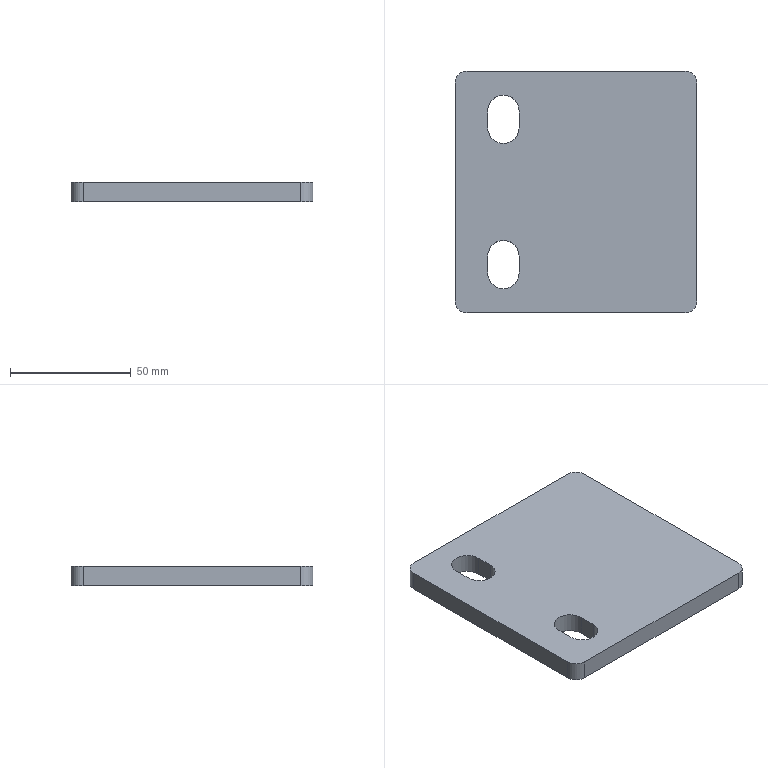Part | STEP file | HL4GD-1.30.104 cab frame rear mounting plate-
-20251212 | 1 solid | 18 faces | box 100 x 100 x 8 mm | volume 76249 mm3 | plane 10 | cylinder 8 | commonest cylinder face diameters 10 x4 13 x4
STEP:
#1=CARTESIAN_POINT('',(0.,0.,0.));
#2=DIRECTION('',(0.,0.,1.));
#3=DIRECTION('',(1.,0.,0.));
#4=AXIS2_PLACEMENT_3D('',#1,#2,#3);
#5=CARTESIAN_POINT('',(1488.5,543.5,1008.452));
#6=VERTEX_POINT('',#5);
#7=CARTESIAN_POINT('',(1488.5,543.5,1000.452));
#8=VERTEX_POINT('',#7);
#9=CARTESIAN_POINT('',(1488.5,543.5,-1016.452));
#10=DIRECTION('',(0.,0.,-1.));
#11=VECTOR('',#10,1.);
#12=LINE('',#9,#11);
#13=CARTESIAN_POINT('',(1495.,543.5,-1016.452));
#14=DIRECTION('',(0.,0.,1.));
#15=DIRECTION('',(0.,1.,0.));
#16=AXIS2_PLACEMENT_3D('',#13,#14,#15);
#17=CYLINDRICAL_SURFACE('',#16,6.5);
#18=CARTESIAN_POINT('',(1.571,0.));
#19=DIRECTION('',(0.,-1.));
#20=VECTOR('',#19,1.);
#21=LINE('',#18,#20);
#22=(GEOMETRIC_REPRESENTATION_CONTEXT(2)PARAMETRIC_REPRESENTATION_CONTEXT()REPRESENTATION_CONTEXT('',''));
#23=DEFINITIONAL_REPRESENTATION('',(#21),#22);
#24=PCURVE('',#17,#23);
#25=CARTESIAN_POINT('',(1488.5,543.5,-1016.452));
#26=DIRECTION('',(1.,0.,0.));
#27=DIRECTION('',(0.,0.,1.));
#28=AXIS2_PLACEMENT_3D('',#25,#26,#27);
#29=PLANE('',#28);
#30=CARTESIAN_POINT('',(0.,0.));
#31=DIRECTION('',(-1.,0.));
#32=VECTOR('',#31,1.);
#33=LINE('',#30,#32);
#34=(GEOMETRIC_REPRESENTATION_CONTEXT(2)PARAMETRIC_REPRESENTATION_CONTEXT()REPRESENTATION_CONTEXT('',''));
#35=DEFINITIONAL_REPRESENTATION('',(#33),#34);
#36=PCURVE('',#29,#35);
#37=SURFACE_CURVE('',#12,(#24,#36),.PCURVE_S1.);
#38=EDGE_CURVE('',#6,#8,#37,.T.);
#39=ORIENTED_EDGE('',*,*,#38,.F.);
#40=CARTESIAN_POINT('',(1501.5,543.5,1008.452));
#41=VERTEX_POINT('',#40);
#42=CARTESIAN_POINT('',(1495.,543.5,1008.452));
#43=DIRECTION('',(0.,0.,-1.));
#44=DIRECTION('',(1.,0.,0.));
#45=AXIS2_PLACEMENT_3D('',#42,#43,#44);
#46=CIRCLE('',#45,6.5);
#47=CARTESIAN_POINT('',(4.712,2024.905));
#48=DIRECTION('',(-1.,0.));
#49=VECTOR('',#48,1.);
#50=LINE('',#47,#49);
#51=(GEOMETRIC_REPRESENTATION_CONTEXT(2)PARAMETRIC_REPRESENTATION_CONTEXT()REPRESENTATION_CONTEXT('',''));
#52=DEFINITIONAL_REPRESENTATION('',(#50),#51);
#53=PCURVE('',#17,#52);
#54=CARTESIAN_POINT('',(1525.,570.,1008.452));
#55=DIRECTION('',(0.,0.,1.));
#56=DIRECTION('',(1.,0.,0.));
#57=AXIS2_PLACEMENT_3D('',#54,#55,#56);
#58=PLANE('',#57);
#59=CARTESIAN_POINT('',(-23.5,-26.5));
#60=CARTESIAN_POINT('',(-23.5,-37.758));
#61=CARTESIAN_POINT('',(-33.25,-32.129));
#62=CARTESIAN_POINT('',(-43.,-26.5));
#63=CARTESIAN_POINT('',(-33.25,-20.871));
#64=CARTESIAN_POINT('',(-23.5,-15.242));
#65=CARTESIAN_POINT('',(-23.5,-26.5));
#66=(BOUNDED_CURVE()B_SPLINE_CURVE(2,(#59,#60,#61,#62,#63,#64,#65),.UNSPECIFIED.,.T.,.F.)B_SPLINE_CURVE_WITH_KNOTS((1,2,2,2,2,1),(-2.094,0.,2.094,4.189,6.283,8.378),.UNSPECIFIED.)CURVE()GEOMETRIC_REPRESENTATION_ITEM()RATIONAL_B_SPLINE_CURVE((1.,0.5,1.,0.5,1.,0.5,1.))REPRESENTATION_ITEM(''));
#67=(GEOMETRIC_REPRESENTATION_CONTEXT(2)PARAMETRIC_REPRESENTATION_CONTEXT()REPRESENTATION_CONTEXT('',''));
#68=DEFINITIONAL_REPRESENTATION('',(#66),#67);
#69=PCURVE('',#58,#68);
#70=SURFACE_CURVE('',#46,(#53,#69),.PCURVE_S1.);
#71=EDGE_CURVE('',#6,#41,#70,.T.);
#72=ORIENTED_EDGE('',*,*,#71,.T.);
#73=CARTESIAN_POINT('',(1501.5,543.5,1000.452));
#74=VERTEX_POINT('',#73);
#75=CARTESIAN_POINT('',(1501.5,543.5,-1016.452));
#76=DIRECTION('',(0.,0.,-1.));
#77=VECTOR('',#76,1.);
#78=LINE('',#75,#77);
#79=CARTESIAN_POINT('',(-1.571,0.));
#80=DIRECTION('',(0.,-1.));
#81=VECTOR('',#80,1.);
#82=LINE('',#79,#81);
#83=(GEOMETRIC_REPRESENTATION_CONTEXT(2)PARAMETRIC_REPRESENTATION_CONTEXT()REPRESENTATION_CONTEXT('',''));
#84=DEFINITIONAL_REPRESENTATION('',(#82),#83);
#85=PCURVE('',#17,#84);
#86=CARTESIAN_POINT('',(1501.5,536.5,-1016.452));
#87=DIRECTION('',(-1.,0.,0.));
#88=DIRECTION('',(0.,0.,-1.));
#89=AXIS2_PLACEMENT_3D('',#86,#87,#88);
#90=PLANE('',#89);
#91=CARTESIAN_POINT('',(0.,-7.));
#92=DIRECTION('',(1.,0.));
#93=VECTOR('',#92,1.);
#94=LINE('',#91,#93);
#95=(GEOMETRIC_REPRESENTATION_CONTEXT(2)PARAMETRIC_REPRESENTATION_CONTEXT()REPRESENTATION_CONTEXT('',''));
#96=DEFINITIONAL_REPRESENTATION('',(#94),#95);
#97=PCURVE('',#90,#96);
#98=SURFACE_CURVE('',#78,(#85,#97),.PCURVE_S1.);
#99=EDGE_CURVE('',#41,#74,#98,.T.);
#100=ORIENTED_EDGE('',*,*,#99,.T.);
#101=CARTESIAN_POINT('',(1495.,543.5,1000.452));
#102=DIRECTION('',(0.,0.,1.));
#103=DIRECTION('',(-1.,0.,0.));
#104=AXIS2_PLACEMENT_3D('',#101,#102,#103);
#105=CIRCLE('',#104,6.5);
#106=CARTESIAN_POINT('',(-4.712,2016.905));
#107=DIRECTION('',(1.,0.));
#108=VECTOR('',#107,1.);
#109=LINE('',#106,#108);
#110=(GEOMETRIC_REPRESENTATION_CONTEXT(2)PARAMETRIC_REPRESENTATION_CONTEXT()REPRESENTATION_CONTEXT('',''));
#111=DEFINITIONAL_REPRESENTATION('',(#109),#110);
#112=PCURVE('',#17,#111);
#113=CARTESIAN_POINT('',(1565.,560.,1000.452));
#114=DIRECTION('',(0.,0.,-1.));
#115=DIRECTION('',(1.,0.,0.));
#116=AXIS2_PLACEMENT_3D('',#113,#114,#115);
#117=PLANE('',#116);
#118=CARTESIAN_POINT('',(-76.5,16.5));
#119=CARTESIAN_POINT('',(-76.5,27.758));
#120=CARTESIAN_POINT('',(-66.75,22.129));
#121=CARTESIAN_POINT('',(-57.,16.5));
#122=CARTESIAN_POINT('',(-66.75,10.871));
#123=CARTESIAN_POINT('',(-76.5,5.242));
#124=CARTESIAN_POINT('',(-76.5,16.5));
#125=(BOUNDED_CURVE()B_SPLINE_CURVE(2,(#118,#119,#120,#121,#122,#123,#124),.UNSPECIFIED.,.T.,.F.)B_SPLINE_CURVE_WITH_KNOTS((1,2,2,2,2,1),(-2.094,0.,2.094,4.189,6.283,8.378),.UNSPECIFIED.)CURVE()GEOMETRIC_REPRESENTATION_ITEM()RATIONAL_B_SPLINE_CURVE((1.,0.5,1.,0.5,1.,0.5,1.))REPRESENTATION_ITEM(''));
#126=(GEOMETRIC_REPRESENTATION_CONTEXT(2)PARAMETRIC_REPRESENTATION_CONTEXT()REPRESENTATION_CONTEXT('',''));
#127=DEFINITIONAL_REPRESENTATION('',(#125),#126);
#128=PCURVE('',#117,#127);
#129=SURFACE_CURVE('',#105,(#112,#128),.PCURVE_S1.);
#130=EDGE_CURVE('',#74,#8,#129,.T.);
#131=ORIENTED_EDGE('',*,*,#130,.T.);
#132=EDGE_LOOP('',(#39,#72,#100,#131));
#133=FACE_BOUND('',#132,.F.);
#134=ADVANCED_FACE('',(#133),#17,.F.);
#135=CARTESIAN_POINT('',(1488.5,536.5,1008.452));
#136=VERTEX_POINT('',#135);
#137=CARTESIAN_POINT('',(1488.5,570.,1008.452));
#138=DIRECTION('',(0.,1.,0.));
#139=VECTOR('',#138,1.);
#140=LINE('',#137,#139);
#141=CARTESIAN_POINT('',(2024.905,-26.5));
#142=DIRECTION('',(0.,-1.));
#143=VECTOR('',#142,1.);
#144=LINE('',#141,#143);
#145=(GEOMETRIC_REPRESENTATION_CONTEXT(2)PARAMETRIC_REPRESENTATION_CONTEXT()REPRESENTATION_CONTEXT('',''));
#146=DEFINITIONAL_REPRESENTATION('',(#144),#145);
#147=PCURVE('',#29,#146);
#148=CARTESIAN_POINT('',(-36.5,0.));
#149=DIRECTION('',(0.,1.));
#150=VECTOR('',#149,1.);
#151=LINE('',#148,#150);
#152=(GEOMETRIC_REPRESENTATION_CONTEXT(2)PARAMETRIC_REPRESENTATION_CONTEXT()REPRESENTATION_CONTEXT('',''));
#153=DEFINITIONAL_REPRESENTATION('',(#151),#152);
#154=PCURVE('',#58,#153);
#155=SURFACE_CURVE('',#140,(#147,#154),.PCURVE_S1.);
#156=EDGE_CURVE('',#136,#6,#155,.T.);
#157=ORIENTED_EDGE('',*,*,#156,.F.);
#158=CARTESIAN_POINT('',(1488.5,536.5,1000.452));
#159=VERTEX_POINT('',#158);
#160=CARTESIAN_POINT('',(1488.5,536.5,-1016.452));
#161=DIRECTION('',(0.,0.,-1.));
#162=VECTOR('',#161,1.);
#163=LINE('',#160,#162);
#164=CARTESIAN_POINT('',(0.,7.));
#165=DIRECTION('',(-1.,0.));
#166=VECTOR('',#165,1.);
#167=LINE('',#164,#166);
#168=(GEOMETRIC_REPRESENTATION_CONTEXT(2)PARAMETRIC_REPRESENTATION_CONTEXT()REPRESENTATION_CONTEXT('',''));
#169=DEFINITIONAL_REPRESENTATION('',(#167),#168);
#170=PCURVE('',#29,#169);
#171=CARTESIAN_POINT('',(1495.,536.5,-1016.452));
#172=DIRECTION('',(0.,0.,1.));
#173=DIRECTION('',(0.,1.,0.));
#174=AXIS2_PLACEMENT_3D('',#171,#172,#173);
#175=CYLINDRICAL_SURFACE('',#174,6.5);
#176=CARTESIAN_POINT('',(1.571,0.));
#177=DIRECTION('',(0.,-1.));
#178=VECTOR('',#177,1.);
#179=LINE('',#176,#178);
#180=(GEOMETRIC_REPRESENTATION_CONTEXT(2)PARAMETRIC_REPRESENTATION_CONTEXT()REPRESENTATION_CONTEXT('',''));
#181=DEFINITIONAL_REPRESENTATION('',(#179),#180);
#182=PCURVE('',#175,#181);
#183=SURFACE_CURVE('',#163,(#170,#182),.PCURVE_S1.);
#184=EDGE_CURVE('',#136,#159,#183,.T.);
#185=ORIENTED_EDGE('',*,*,#184,.T.);
#186=CARTESIAN_POINT('',(1488.5,560.,1000.452));
#187=DIRECTION('',(0.,-1.,0.));
#188=VECTOR('',#187,1.);
#189=LINE('',#186,#188);
#190=CARTESIAN_POINT('',(2016.905,-16.5));
#191=DIRECTION('',(0.,1.));
#192=VECTOR('',#191,1.);
#193=LINE('',#190,#192);
#194=(GEOMETRIC_REPRESENTATION_CONTEXT(2)PARAMETRIC_REPRESENTATION_CONTEXT()REPRESENTATION_CONTEXT('',''));
#195=DEFINITIONAL_REPRESENTATION('',(#193),#194);
#196=PCURVE('',#29,#195);
#197=CARTESIAN_POINT('',(-76.5,0.));
#198=DIRECTION('',(0.,1.));
#199=VECTOR('',#198,1.);
#200=LINE('',#197,#199);
#201=(GEOMETRIC_REPRESENTATION_CONTEXT(2)PARAMETRIC_REPRESENTATION_CONTEXT()REPRESENTATION_CONTEXT('',''));
#202=DEFINITIONAL_REPRESENTATION('',(#200),#201);
#203=PCURVE('',#117,#202);
#204=SURFACE_CURVE('',#189,(#196,#203),.PCURVE_S1.);
#205=EDGE_CURVE('',#8,#159,#204,.T.);
#206=ORIENTED_EDGE('',*,*,#205,.F.);
#207=ORIENTED_EDGE('',*,*,#38,.F.);
#208=EDGE_LOOP('',(#157,#185,#206,#207));
#209=FACE_BOUND('',#208,.T.);
#210=ADVANCED_FACE('',(#209),#29,.T.);
#211=CARTESIAN_POINT('',(1501.5,536.5,1008.452));
#212=VERTEX_POINT('',#211);
#213=CARTESIAN_POINT('',(1501.5,536.5,1000.452));
#214=VERTEX_POINT('',#213);
#215=CARTESIAN_POINT('',(1501.5,536.5,-1016.452));
#216=DIRECTION('',(0.,0.,-1.));
#217=VECTOR('',#216,1.);
#218=LINE('',#215,#217);
#219=CARTESIAN_POINT('',(4.712,0.));
#220=DIRECTION('',(0.,-1.));
#221=VECTOR('',#220,1.);
#222=LINE('',#219,#221);
#223=(GEOMETRIC_REPRESENTATION_CONTEXT(2)PARAMETRIC_REPRESENTATION_CONTEXT()REPRESENTATION_CONTEXT('',''));
#224=DEFINITIONAL_REPRESENTATION('',(#222),#223);
#225=PCURVE('',#175,#224);
#226=CARTESIAN_POINT('',(0.,0.));
#227=DIRECTION('',(1.,0.));
#228=VECTOR('',#227,1.);
#229=LINE('',#226,#228);
#230=(GEOMETRIC_REPRESENTATION_CONTEXT(2)PARAMETRIC_REPRESENTATION_CONTEXT()REPRESENTATION_CONTEXT('',''));
#231=DEFINITIONAL_REPRESENTATION('',(#229),#230);
#232=PCURVE('',#90,#231);
#233=SURFACE_CURVE('',#218,(#225,#232),.PCURVE_S1.);
#234=EDGE_CURVE('',#212,#214,#233,.T.);
#235=ORIENTED_EDGE('',*,*,#234,.F.);
#236=CARTESIAN_POINT('',(1495.,536.5,1008.452));
#237=DIRECTION('',(0.,0.,-1.));
#238=DIRECTION('',(1.,0.,0.));
#239=AXIS2_PLACEMENT_3D('',#236,#237,#238);
#240=CIRCLE('',#239,6.5);
#241=CARTESIAN_POINT('',(4.712,2024.905));
#242=DIRECTION('',(-1.,0.));
#243=VECTOR('',#242,1.);
#244=LINE('',#241,#243);
#245=(GEOMETRIC_REPRESENTATION_CONTEXT(2)PARAMETRIC_REPRESENTATION_CONTEXT()REPRESENTATION_CONTEXT('',''));
#246=DEFINITIONAL_REPRESENTATION('',(#244),#245);
#247=PCURVE('',#175,#246);
#248=CARTESIAN_POINT('',(-23.5,-33.5));
#249=CARTESIAN_POINT('',(-23.5,-44.758));
#250=CARTESIAN_POINT('',(-33.25,-39.129));
#251=CARTESIAN_POINT('',(-43.,-33.5));
#252=CARTESIAN_POINT('',(-33.25,-27.871));
#253=CARTESIAN_POINT('',(-23.5,-22.242));
#254=CARTESIAN_POINT('',(-23.5,-33.5));
#255=(BOUNDED_CURVE()B_SPLINE_CURVE(2,(#248,#249,#250,#251,#252,#253,#254),.UNSPECIFIED.,.T.,.F.)B_SPLINE_CURVE_WITH_KNOTS((1,2,2,2,2,1),(-2.094,0.,2.094,4.189,6.283,8.378),.UNSPECIFIED.)CURVE()GEOMETRIC_REPRESENTATION_ITEM()RATIONAL_B_SPLINE_CURVE((1.,0.5,1.,0.5,1.,0.5,1.))REPRESENTATION_ITEM(''));
#256=(GEOMETRIC_REPRESENTATION_CONTEXT(2)PARAMETRIC_REPRESENTATION_CONTEXT()REPRESENTATION_CONTEXT('',''));
#257=DEFINITIONAL_REPRESENTATION('',(#255),#256);
#258=PCURVE('',#58,#257);
#259=SURFACE_CURVE('',#240,(#247,#258),.PCURVE_S1.);
#260=EDGE_CURVE('',#212,#136,#259,.T.);
#261=ORIENTED_EDGE('',*,*,#260,.T.);
#262=ORIENTED_EDGE('',*,*,#184,.T.);
#263=CARTESIAN_POINT('',(1495.,536.5,1000.452));
#264=DIRECTION('',(0.,0.,1.));
#265=DIRECTION('',(-1.,0.,0.));
#266=AXIS2_PLACEMENT_3D('',#263,#264,#265);
#267=CIRCLE('',#266,6.5);
#268=CARTESIAN_POINT('',(1.571,2016.905));
#269=DIRECTION('',(1.,0.));
#270=VECTOR('',#269,1.);
#271=LINE('',#268,#270);
#272=(GEOMETRIC_REPRESENTATION_CONTEXT(2)PARAMETRIC_REPRESENTATION_CONTEXT()REPRESENTATION_CONTEXT('',''));
#273=DEFINITIONAL_REPRESENTATION('',(#271),#272);
#274=PCURVE('',#175,#273);
#275=CARTESIAN_POINT('',(-76.5,23.5));
#276=CARTESIAN_POINT('',(-76.5,34.758));
#277=CARTESIAN_POINT('',(-66.75,29.129));
#278=CARTESIAN_POINT('',(-57.,23.5));
#279=CARTESIAN_POINT('',(-66.75,17.871));
#280=CARTESIAN_POINT('',(-76.5,12.242));
#281=CARTESIAN_POINT('',(-76.5,23.5));
#282=(BOUNDED_CURVE()B_SPLINE_CURVE(2,(#275,#276,#277,#278,#279,#280,#281),.UNSPECIFIED.,.T.,.F.)B_SPLINE_CURVE_WITH_KNOTS((1,2,2,2,2,1),(-2.094,0.,2.094,4.189,6.283,8.378),.UNSPECIFIED.)CURVE()GEOMETRIC_REPRESENTATION_ITEM()RATIONAL_B_SPLINE_CURVE((1.,0.5,1.,0.5,1.,0.5,1.))REPRESENTATION_ITEM(''));
#283=(GEOMETRIC_REPRESENTATION_CONTEXT(2)PARAMETRIC_REPRESENTATION_CONTEXT()REPRESENTATION_CONTEXT('',''));
#284=DEFINITIONAL_REPRESENTATION('',(#282),#283);
#285=PCURVE('',#117,#284);
#286=SURFACE_CURVE('',#267,(#274,#285),.PCURVE_S1.);
#287=EDGE_CURVE('',#159,#214,#286,.T.);
#288=ORIENTED_EDGE('',*,*,#287,.T.);
#289=EDGE_LOOP('',(#235,#261,#262,#288));
#290=FACE_BOUND('',#289,.F.);
#291=ADVANCED_FACE('',(#290),#175,.F.);
#292=CARTESIAN_POINT('',(1501.5,570.,1008.452));
#293=DIRECTION('',(0.,-1.,0.));
#294=VECTOR('',#293,1.);
#295=LINE('',#292,#294);
#296=CARTESIAN_POINT('',(-2024.905,-33.5));
#297=DIRECTION('',(0.,1.));
#298=VECTOR('',#297,1.);
#299=LINE('',#296,#298);
#300=(GEOMETRIC_REPRESENTATION_CONTEXT(2)PARAMETRIC_REPRESENTATION_CONTEXT()REPRESENTATION_CONTEXT('',''));
#301=DEFINITIONAL_REPRESENTATION('',(#299),#300);
#302=PCURVE('',#90,#301);
#303=CARTESIAN_POINT('',(-23.5,0.));
#304=DIRECTION('',(0.,-1.));
#305=VECTOR('',#304,1.);
#306=LINE('',#303,#305);
#307=(GEOMETRIC_REPRESENTATION_CONTEXT(2)PARAMETRIC_REPRESENTATION_CONTEXT()REPRESENTATION_CONTEXT('',''));
#308=DEFINITIONAL_REPRESENTATION('',(#306),#307);
#309=PCURVE('',#58,#308);
#310=SURFACE_CURVE('',#295,(#302,#309),.PCURVE_S1.);
#311=EDGE_CURVE('',#41,#212,#310,.T.);
#312=ORIENTED_EDGE('',*,*,#311,.F.);
#313=ORIENTED_EDGE('',*,*,#99,.T.);
#314=CARTESIAN_POINT('',(1501.5,560.,1000.452));
#315=DIRECTION('',(0.,1.,0.));
#316=VECTOR('',#315,1.);
#317=LINE('',#314,#316);
#318=CARTESIAN_POINT('',(-2016.905,-23.5));
#319=DIRECTION('',(0.,-1.));
#320=VECTOR('',#319,1.);
#321=LINE('',#318,#320);
#322=(GEOMETRIC_REPRESENTATION_CONTEXT(2)PARAMETRIC_REPRESENTATION_CONTEXT()REPRESENTATION_CONTEXT('',''));
#323=DEFINITIONAL_REPRESENTATION('',(#321),#322);
#324=PCURVE('',#90,#323);
#325=CARTESIAN_POINT('',(-63.5,0.));
#326=DIRECTION('',(0.,-1.));
#327=VECTOR('',#326,1.);
#328=LINE('',#325,#327);
#329=(GEOMETRIC_REPRESENTATION_CONTEXT(2)PARAMETRIC_REPRESENTATION_CONTEXT()REPRESENTATION_CONTEXT('',''));
#330=DEFINITIONAL_REPRESENTATION('',(#328),#329);
#331=PCURVE('',#117,#330);
#332=SURFACE_CURVE('',#317,(#324,#331),.PCURVE_S1.);
#333=EDGE_CURVE('',#214,#74,#332,.T.);
#334=ORIENTED_EDGE('',*,*,#333,.F.);
#335=ORIENTED_EDGE('',*,*,#234,.F.);
#336=EDGE_LOOP('',(#312,#313,#334,#335));
#337=FACE_BOUND('',#336,.T.);
#338=ADVANCED_FACE('',(#337),#90,.T.);
#339=CARTESIAN_POINT('',(1501.5,603.5,1000.452));
#340=VERTEX_POINT('',#339);
#341=CARTESIAN_POINT('',(1501.5,596.5,1000.452));
#342=VERTEX_POINT('',#341);
#343=CARTESIAN_POINT('',(1501.5,530.,1000.452));
#344=DIRECTION('',(0.,-1.,0.));
#345=VECTOR('',#344,1.);
#346=LINE('',#343,#345);
#347=CARTESIAN_POINT('',(-63.5,30.));
#348=DIRECTION('',(0.,1.));
#349=VECTOR('',#348,1.);
#350=LINE('',#347,#349);
#351=(GEOMETRIC_REPRESENTATION_CONTEXT(2)PARAMETRIC_REPRESENTATION_CONTEXT()REPRESENTATION_CONTEXT('',''));
#352=DEFINITIONAL_REPRESENTATION('',(#350),#351);
#353=PCURVE('',#117,#352);
#354=CARTESIAN_POINT('',(1501.5,603.5,-1016.452));
#355=DIRECTION('',(-1.,0.,0.));
#356=DIRECTION('',(0.,0.,-1.));
#357=AXIS2_PLACEMENT_3D('',#354,#355,#356);
#358=PLANE('',#357);
#359=CARTESIAN_POINT('',(-2016.905,73.5));
#360=DIRECTION('',(0.,1.));
#361=VECTOR('',#360,1.);
#362=LINE('',#359,#361);
#363=(GEOMETRIC_REPRESENTATION_CONTEXT(2)PARAMETRIC_REPRESENTATION_CONTEXT()REPRESENTATION_CONTEXT('',''));
#364=DEFINITIONAL_REPRESENTATION('',(#362),#363);
#365=PCURVE('',#358,#364);
#366=SURFACE_CURVE('',#346,(#353,#365),.PCURVE_S1.);
#367=EDGE_CURVE('',#340,#342,#366,.T.);
#368=ORIENTED_EDGE('',*,*,#367,.F.);
#369=CARTESIAN_POINT('',(1488.5,603.5,1000.452));
#370=VERTEX_POINT('',#369);
#371=CARTESIAN_POINT('',(1495.,603.5,1000.452));
#372=DIRECTION('',(0.,0.,-1.));
#373=DIRECTION('',(0.,1.,0.));
#374=AXIS2_PLACEMENT_3D('',#371,#372,#373);
#375=CIRCLE('',#374,6.5);
#376=CARTESIAN_POINT('',(-70.,-43.5));
#377=DIRECTION('',(0.,-1.));
#378=AXIS2_PLACEMENT_2D('',#376,#377);
#379=CIRCLE('',#378,6.5);
#380=(GEOMETRIC_REPRESENTATION_CONTEXT(2)PARAMETRIC_REPRESENTATION_CONTEXT()REPRESENTATION_CONTEXT('',''));
#381=DEFINITIONAL_REPRESENTATION('',(#379),#380);
#382=PCURVE('',#117,#381);
#383=CARTESIAN_POINT('',(1495.,603.5,-1016.452));
#384=DIRECTION('',(0.,0.,1.));
#385=DIRECTION('',(0.,-1.,0.));
#386=AXIS2_PLACEMENT_3D('',#383,#384,#385);
#387=CYLINDRICAL_SURFACE('',#386,6.5);
#388=CARTESIAN_POINT('',(9.425,2016.905));
#389=DIRECTION('',(-1.,0.));
#390=VECTOR('',#389,1.);
#391=LINE('',#388,#390);
#392=(GEOMETRIC_REPRESENTATION_CONTEXT(2)PARAMETRIC_REPRESENTATION_CONTEXT()REPRESENTATION_CONTEXT('',''));
#393=DEFINITIONAL_REPRESENTATION('',(#391),#392);
#394=PCURVE('',#387,#393);
#395=SURFACE_CURVE('',#375,(#382,#394),.PCURVE_S1.);
#396=EDGE_CURVE('',#370,#340,#395,.T.);
#397=ORIENTED_EDGE('',*,*,#396,.F.);
#398=CARTESIAN_POINT('',(1488.5,596.5,1000.452));
#399=VERTEX_POINT('',#398);
#400=CARTESIAN_POINT('',(1488.5,530.,1000.452));
#401=DIRECTION('',(0.,1.,0.));
#402=VECTOR('',#401,1.);
#403=LINE('',#400,#402);
#404=CARTESIAN_POINT('',(-76.5,30.));
#405=DIRECTION('',(0.,-1.));
#406=VECTOR('',#405,1.);
#407=LINE('',#404,#406);
#408=(GEOMETRIC_REPRESENTATION_CONTEXT(2)PARAMETRIC_REPRESENTATION_CONTEXT()REPRESENTATION_CONTEXT('',''));
#409=DEFINITIONAL_REPRESENTATION('',(#407),#408);
#410=PCURVE('',#117,#409);
#411=CARTESIAN_POINT('',(1488.5,596.5,-1016.452));
#412=DIRECTION('',(1.,0.,0.));
#413=DIRECTION('',(0.,0.,1.));
#414=AXIS2_PLACEMENT_3D('',#411,#412,#413);
#415=PLANE('',#414);
#416=CARTESIAN_POINT('',(2016.905,66.5));
#417=DIRECTION('',(0.,-1.));
#418=VECTOR('',#417,1.);
#419=LINE('',#416,#418);
#420=(GEOMETRIC_REPRESENTATION_CONTEXT(2)PARAMETRIC_REPRESENTATION_CONTEXT()REPRESENTATION_CONTEXT('',''));
#421=DEFINITIONAL_REPRESENTATION('',(#419),#420);
#422=PCURVE('',#415,#421);
#423=SURFACE_CURVE('',#403,(#410,#422),.PCURVE_S1.);
#424=EDGE_CURVE('',#399,#370,#423,.T.);
#425=ORIENTED_EDGE('',*,*,#424,.F.);
#426=CARTESIAN_POINT('',(1495.,596.5,1000.452));
#427=DIRECTION('',(0.,0.,1.));
#428=DIRECTION('',(0.,1.,0.));
#429=AXIS2_PLACEMENT_3D('',#426,#427,#428);
#430=CIRCLE('',#429,6.5);
#431=CARTESIAN_POINT('',(-70.,-43.));
#432=CARTESIAN_POINT('',(-81.258,-43.));
#433=CARTESIAN_POINT('',(-75.629,-33.25));
#434=CARTESIAN_POINT('',(-70.,-23.5));
#435=CARTESIAN_POINT('',(-64.371,-33.25));
#436=CARTESIAN_POINT('',(-58.742,-43.));
#437=CARTESIAN_POINT('',(-70.,-43.));
#438=(BOUNDED_CURVE()B_SPLINE_CURVE(2,(#431,#432,#433,#434,#435,#436,#437),.UNSPECIFIED.,.T.,.F.)B_SPLINE_CURVE_WITH_KNOTS((1,2,2,2,2,1),(-2.094,0.,2.094,4.189,6.283,8.378),.UNSPECIFIED.)CURVE()GEOMETRIC_REPRESENTATION_ITEM()RATIONAL_B_SPLINE_CURVE((1.,0.5,1.,0.5,1.,0.5,1.))REPRESENTATION_ITEM(''));
#439=(GEOMETRIC_REPRESENTATION_CONTEXT(2)PARAMETRIC_REPRESENTATION_CONTEXT()REPRESENTATION_CONTEXT('',''));
#440=DEFINITIONAL_REPRESENTATION('',(#438),#439);
#441=PCURVE('',#117,#440);
#442=CARTESIAN_POINT('',(1495.,596.5,-1016.452));
#443=DIRECTION('',(0.,0.,1.));
#444=DIRECTION('',(0.,-1.,0.));
#445=AXIS2_PLACEMENT_3D('',#442,#443,#444);
#446=CYLINDRICAL_SURFACE('',#445,6.5);
#447=CARTESIAN_POINT('',(-3.142,2016.905));
#448=DIRECTION('',(1.,0.));
#449=VECTOR('',#448,1.);
#450=LINE('',#447,#449);
#451=(GEOMETRIC_REPRESENTATION_CONTEXT(2)PARAMETRIC_REPRESENTATION_CONTEXT()REPRESENTATION_CONTEXT('',''));
#452=DEFINITIONAL_REPRESENTATION('',(#450),#451);
#453=PCURVE('',#446,#452);
#454=SURFACE_CURVE('',#430,(#441,#453),.PCURVE_S1.);
#455=EDGE_CURVE('',#399,#342,#454,.T.);
#456=ORIENTED_EDGE('',*,*,#455,.T.);
#457=EDGE_LOOP('',(#368,#397,#425,#456));
#458=FACE_BOUND('',#457,.T.);
#459=CARTESIAN_POINT('',(1575.,525.,1000.452));
#460=VERTEX_POINT('',#459);
#461=CARTESIAN_POINT('',(1575.,615.,1000.452));
#462=VERTEX_POINT('',#461);
#463=CARTESIAN_POINT('',(1575.,560.,1000.452));
#464=DIRECTION('',(0.,1.,0.));
#465=VECTOR('',#464,1.);
#466=LINE('',#463,#465);
#467=CARTESIAN_POINT('',(10.,0.));
#468=DIRECTION('',(0.,-1.));
#469=VECTOR('',#468,1.);
#470=LINE('',#467,#469);
#471=(GEOMETRIC_REPRESENTATION_CONTEXT(2)PARAMETRIC_REPRESENTATION_CONTEXT()REPRESENTATION_CONTEXT('',''));
#472=DEFINITIONAL_REPRESENTATION('',(#470),#471);
#473=PCURVE('',#117,#472);
#474=CARTESIAN_POINT('',(1575.,560.,1425.));
#475=DIRECTION('',(1.,0.,0.));
#476=DIRECTION('',(0.,0.,1.));
#477=AXIS2_PLACEMENT_3D('',#474,#475,#476);
#478=PLANE('',#477);
#479=CARTESIAN_POINT('',(-424.548,0.));
#480=DIRECTION('',(0.,-1.));
#481=VECTOR('',#480,1.);
#482=LINE('',#479,#481);
#483=(GEOMETRIC_REPRESENTATION_CONTEXT(2)PARAMETRIC_REPRESENTATION_CONTEXT()REPRESENTATION_CONTEXT('',''));
#484=DEFINITIONAL_REPRESENTATION('',(#482),#483);
#485=PCURVE('',#478,#484);
#486=SURFACE_CURVE('',#466,(#473,#485),.PCURVE_S1.);
#487=EDGE_CURVE('',#460,#462,#486,.T.);
#488=ORIENTED_EDGE('',*,*,#487,.F.);
#489=CARTESIAN_POINT('',(1570.,520.,1000.452));
#490=VERTEX_POINT('',#489);
#491=CARTESIAN_POINT('',(1570.,525.,1000.452));
#492=DIRECTION('',(0.,0.,-1.));
#493=DIRECTION('',(-1.,0.,0.));
#494=AXIS2_PLACEMENT_3D('',#491,#492,#493);
#495=CIRCLE('',#494,5.);
#496=CARTESIAN_POINT('',(5.,35.));
#497=DIRECTION('',(-1.,0.));
#498=AXIS2_PLACEMENT_2D('',#496,#497);
#499=CIRCLE('',#498,5.);
#500=(GEOMETRIC_REPRESENTATION_CONTEXT(2)PARAMETRIC_REPRESENTATION_CONTEXT()REPRESENTATION_CONTEXT('',''));
#501=DEFINITIONAL_REPRESENTATION('',(#499),#500);
#502=PCURVE('',#117,#501);
#503=CARTESIAN_POINT('',(1570.,525.,1425.));
#504=DIRECTION('',(0.,0.,1.));
#505=DIRECTION('',(1.,0.,0.));
#506=AXIS2_PLACEMENT_3D('',#503,#504,#505);
#507=CYLINDRICAL_SURFACE('',#506,5.);
#508=CARTESIAN_POINT('',(9.425,-424.548));
#509=DIRECTION('',(-1.,0.));
#510=VECTOR('',#509,1.);
#511=LINE('',#508,#510);
#512=(GEOMETRIC_REPRESENTATION_CONTEXT(2)PARAMETRIC_REPRESENTATION_CONTEXT()REPRESENTATION_CONTEXT('',''));
#513=DEFINITIONAL_REPRESENTATION('',(#511),#512);
#514=PCURVE('',#507,#513);
#515=SURFACE_CURVE('',#495,(#502,#514),.PCURVE_S1.);
#516=EDGE_CURVE('',#460,#490,#515,.T.);
#517=ORIENTED_EDGE('',*,*,#516,.T.);
#518=CARTESIAN_POINT('',(1480.,520.,1000.452));
#519=VERTEX_POINT('',#518);
#520=CARTESIAN_POINT('',(1565.,520.,1000.452));
#521=DIRECTION('',(-1.,0.,0.));
#522=VECTOR('',#521,1.);
#523=LINE('',#520,#522);
#524=CARTESIAN_POINT('',(0.,40.));
#525=DIRECTION('',(-1.,0.));
#526=VECTOR('',#525,1.);
#527=LINE('',#524,#526);
#528=(GEOMETRIC_REPRESENTATION_CONTEXT(2)PARAMETRIC_REPRESENTATION_CONTEXT()REPRESENTATION_CONTEXT('',''));
#529=DEFINITIONAL_REPRESENTATION('',(#527),#528);
#530=PCURVE('',#117,#529);
#531=CARTESIAN_POINT('',(1565.,520.,1425.));
#532=DIRECTION('',(0.,-1.,0.));
#533=DIRECTION('',(1.,0.,0.));
#534=AXIS2_PLACEMENT_3D('',#531,#532,#533);
#535=PLANE('',#534);
#536=CARTESIAN_POINT('',(0.,-424.548));
#537=DIRECTION('',(-1.,0.));
#538=VECTOR('',#537,1.);
#539=LINE('',#536,#538);
#540=(GEOMETRIC_REPRESENTATION_CONTEXT(2)PARAMETRIC_REPRESENTATION_CONTEXT()REPRESENTATION_CONTEXT('',''));
#541=DEFINITIONAL_REPRESENTATION('',(#539),#540);
#542=PCURVE('',#535,#541);
#543=SURFACE_CURVE('',#523,(#530,#542),.PCURVE_S1.);
#544=EDGE_CURVE('',#490,#519,#543,.T.);
#545=ORIENTED_EDGE('',*,*,#544,.T.);
#546=CARTESIAN_POINT('',(1475.,525.,1000.452));
#547=VERTEX_POINT('',#546);
#548=CARTESIAN_POINT('',(1480.,525.,1000.452));
#549=DIRECTION('',(0.,0.,-1.));
#550=DIRECTION('',(-1.,0.,0.));
#551=AXIS2_PLACEMENT_3D('',#548,#549,#550);
#552=CIRCLE('',#551,5.);
#553=CARTESIAN_POINT('',(-85.,35.));
#554=DIRECTION('',(-1.,0.));
#555=AXIS2_PLACEMENT_2D('',#553,#554);
#556=CIRCLE('',#555,5.);
#557=(GEOMETRIC_REPRESENTATION_CONTEXT(2)PARAMETRIC_REPRESENTATION_CONTEXT()REPRESENTATION_CONTEXT('',''));
#558=DEFINITIONAL_REPRESENTATION('',(#556),#557);
#559=PCURVE('',#117,#558);
#560=CARTESIAN_POINT('',(1480.,525.,1425.));
#561=DIRECTION('',(0.,0.,-1.));
#562=DIRECTION('',(-1.,0.,0.));
#563=AXIS2_PLACEMENT_3D('',#560,#561,#562);
#564=CYLINDRICAL_SURFACE('',#563,5.);
#565=CARTESIAN_POINT('',(0.,424.548));
#566=DIRECTION('',(1.,0.));
#567=VECTOR('',#566,1.);
#568=LINE('',#565,#567);
#569=(GEOMETRIC_REPRESENTATION_CONTEXT(2)PARAMETRIC_REPRESENTATION_CONTEXT()REPRESENTATION_CONTEXT('',''));
#570=DEFINITIONAL_REPRESENTATION('',(#568),#569);
#571=PCURVE('',#564,#570);
#572=SURFACE_CURVE('',#552,(#559,#571),.PCURVE_S1.);
#573=EDGE_CURVE('',#519,#547,#572,.T.);
#574=ORIENTED_EDGE('',*,*,#573,.T.);
#575=CARTESIAN_POINT('',(1475.,615.,1000.452));
#576=VERTEX_POINT('',#575);
#577=CARTESIAN_POINT('',(1475.,560.,1000.452));
#578=DIRECTION('',(0.,1.,0.));
#579=VECTOR('',#578,1.);
#580=LINE('',#577,#579);
#581=CARTESIAN_POINT('',(-90.,0.));
#582=DIRECTION('',(0.,-1.));
#583=VECTOR('',#582,1.);
#584=LINE('',#581,#583);
#585=(GEOMETRIC_REPRESENTATION_CONTEXT(2)PARAMETRIC_REPRESENTATION_CONTEXT()REPRESENTATION_CONTEXT('',''));
#586=DEFINITIONAL_REPRESENTATION('',(#584),#585);
#587=PCURVE('',#117,#586);
#588=CARTESIAN_POINT('',(1475.,560.,1425.));
#589=DIRECTION('',(1.,0.,0.));
#590=DIRECTION('',(0.,0.,1.));
#591=AXIS2_PLACEMENT_3D('',#588,#589,#590);
#592=PLANE('',#591);
#593=CARTESIAN_POINT('',(-424.548,0.));
#594=DIRECTION('',(0.,-1.));
#595=VECTOR('',#594,1.);
#596=LINE('',#593,#595);
#597=(GEOMETRIC_REPRESENTATION_CONTEXT(2)PARAMETRIC_REPRESENTATION_CONTEXT()REPRESENTATION_CONTEXT('',''));
#598=DEFINITIONAL_REPRESENTATION('',(#596),#597);
#599=PCURVE('',#592,#598);
#600=SURFACE_CURVE('',#580,(#587,#599),.PCURVE_S1.);
#601=EDGE_CURVE('',#547,#576,#600,.T.);
#602=ORIENTED_EDGE('',*,*,#601,.T.);
#603=CARTESIAN_POINT('',(1480.,620.,1000.452));
#604=VERTEX_POINT('',#603);
#605=CARTESIAN_POINT('',(1480.,615.,1000.452));
#606=DIRECTION('',(0.,0.,-1.));
#607=DIRECTION('',(-1.,0.,0.));
#608=AXIS2_PLACEMENT_3D('',#605,#606,#607);
#609=CIRCLE('',#608,5.);
#610=CARTESIAN_POINT('',(-85.,-55.));
#611=DIRECTION('',(-1.,0.));
#612=AXIS2_PLACEMENT_2D('',#610,#611);
#613=CIRCLE('',#612,5.);
#614=(GEOMETRIC_REPRESENTATION_CONTEXT(2)PARAMETRIC_REPRESENTATION_CONTEXT()REPRESENTATION_CONTEXT('',''));
#615=DEFINITIONAL_REPRESENTATION('',(#613),#614);
#616=PCURVE('',#117,#615);
#617=CARTESIAN_POINT('',(1480.,615.,1425.));
#618=DIRECTION('',(0.,0.,1.));
#619=DIRECTION('',(1.,0.,0.));
#620=AXIS2_PLACEMENT_3D('',#617,#618,#619);
#621=CYLINDRICAL_SURFACE('',#620,5.);
#622=CARTESIAN_POINT('',(3.142,-424.548));
#623=DIRECTION('',(-1.,0.));
#624=VECTOR('',#623,1.);
#625=LINE('',#622,#624);
#626=(GEOMETRIC_REPRESENTATION_CONTEXT(2)PARAMETRIC_REPRESENTATION_CONTEXT()REPRESENTATION_CONTEXT('',''));
#627=DEFINITIONAL_REPRESENTATION('',(#625),#626);
#628=PCURVE('',#621,#627);
#629=SURFACE_CURVE('',#609,(#616,#628),.PCURVE_S1.);
#630=EDGE_CURVE('',#576,#604,#629,.T.);
#631=ORIENTED_EDGE('',*,*,#630,.T.);
#632=CARTESIAN_POINT('',(1570.,620.,1000.452));
#633=VERTEX_POINT('',#632);
#634=CARTESIAN_POINT('',(1565.,620.,1000.452));
#635=DIRECTION('',(-1.,0.,0.));
#636=VECTOR('',#635,1.);
#637=LINE('',#634,#636);
#638=CARTESIAN_POINT('',(0.,-60.));
#639=DIRECTION('',(-1.,0.));
#640=VECTOR('',#639,1.);
#641=LINE('',#638,#640);
#642=(GEOMETRIC_REPRESENTATION_CONTEXT(2)PARAMETRIC_REPRESENTATION_CONTEXT()REPRESENTATION_CONTEXT('',''));
#643=DEFINITIONAL_REPRESENTATION('',(#641),#642);
#644=PCURVE('',#117,#643);
#645=CARTESIAN_POINT('',(1565.,620.,1425.));
#646=DIRECTION('',(0.,-1.,0.));
#647=DIRECTION('',(1.,0.,0.));
#648=AXIS2_PLACEMENT_3D('',#645,#646,#647);
#649=PLANE('',#648);
#650=CARTESIAN_POINT('',(0.,-424.548));
#651=DIRECTION('',(-1.,0.));
#652=VECTOR('',#651,1.);
#653=LINE('',#650,#652);
#654=(GEOMETRIC_REPRESENTATION_CONTEXT(2)PARAMETRIC_REPRESENTATION_CONTEXT()REPRESENTATION_CONTEXT('',''));
#655=DEFINITIONAL_REPRESENTATION('',(#653),#654);
#656=PCURVE('',#649,#655);
#657=SURFACE_CURVE('',#637,(#644,#656),.PCURVE_S1.);
#658=EDGE_CURVE('',#633,#604,#657,.T.);
#659=ORIENTED_EDGE('',*,*,#658,.F.);
#660=CARTESIAN_POINT('',(1570.,615.,1000.452));
#661=DIRECTION('',(0.,0.,-1.));
#662=DIRECTION('',(-1.,0.,0.));
#663=AXIS2_PLACEMENT_3D('',#660,#661,#662);
#664=CIRCLE('',#663,5.);
#665=CARTESIAN_POINT('',(5.,-55.));
#666=DIRECTION('',(-1.,0.));
#667=AXIS2_PLACEMENT_2D('',#665,#666);
#668=CIRCLE('',#667,5.);
#669=(GEOMETRIC_REPRESENTATION_CONTEXT(2)PARAMETRIC_REPRESENTATION_CONTEXT()REPRESENTATION_CONTEXT('',''));
#670=DEFINITIONAL_REPRESENTATION('',(#668),#669);
#671=PCURVE('',#117,#670);
#672=CARTESIAN_POINT('',(1570.,615.,1425.));
#673=DIRECTION('',(0.,0.,-1.));
#674=DIRECTION('',(-1.,0.,0.));
#675=AXIS2_PLACEMENT_3D('',#672,#673,#674);
#676=CYLINDRICAL_SURFACE('',#675,5.);
#677=CARTESIAN_POINT('',(0.,424.548));
#678=DIRECTION('',(1.,0.));
#679=VECTOR('',#678,1.);
#680=LINE('',#677,#679);
#681=(GEOMETRIC_REPRESENTATION_CONTEXT(2)PARAMETRIC_REPRESENTATION_CONTEXT()REPRESENTATION_CONTEXT('',''));
#682=DEFINITIONAL_REPRESENTATION('',(#680),#681);
#683=PCURVE('',#676,#682);
#684=SURFACE_CURVE('',#664,(#671,#683),.PCURVE_S1.);
#685=EDGE_CURVE('',#633,#462,#684,.T.);
#686=ORIENTED_EDGE('',*,*,#685,.T.);
#687=EDGE_LOOP('',(#488,#517,#545,#574,#602,#631,#659,#686));
#688=FACE_BOUND('',#687,.T.);
#689=ORIENTED_EDGE('',*,*,#333,.T.);
#690=ORIENTED_EDGE('',*,*,#130,.T.);
#691=ORIENTED_EDGE('',*,*,#205,.T.);
#692=ORIENTED_EDGE('',*,*,#287,.T.);
#693=EDGE_LOOP('',(#689,#690,#691,#692));
#694=FACE_BOUND('',#693,.T.);
#695=ADVANCED_FACE('',(#458,#688,#694),#117,.T.);
#696=CARTESIAN_POINT('',(1501.5,596.5,1008.452));
#697=VERTEX_POINT('',#696);
#698=CARTESIAN_POINT('',(1488.5,596.5,1008.452));
#699=VERTEX_POINT('',#698);
#700=CARTESIAN_POINT('',(1495.,596.5,1008.452));
#701=DIRECTION('',(0.,0.,-1.));
#702=DIRECTION('',(0.,-1.,0.));
#703=AXIS2_PLACEMENT_3D('',#700,#701,#702);
#704=CIRCLE('',#703,6.5);
#705=CARTESIAN_POINT('',(-30.,20.));
#706=CARTESIAN_POINT('',(-41.258,20.));
#707=CARTESIAN_POINT('',(-35.629,29.75));
#708=CARTESIAN_POINT('',(-30.,39.5));
#709=CARTESIAN_POINT('',(-24.371,29.75));
#710=CARTESIAN_POINT('',(-18.742,20.));
#711=CARTESIAN_POINT('',(-30.,20.));
#712=(BOUNDED_CURVE()B_SPLINE_CURVE(2,(#705,#706,#707,#708,#709,#710,#711),.UNSPECIFIED.,.T.,.F.)B_SPLINE_CURVE_WITH_KNOTS((1,2,2,2,2,1),(-2.094,0.,2.094,4.189,6.283,8.378),.UNSPECIFIED.)CURVE()GEOMETRIC_REPRESENTATION_ITEM()RATIONAL_B_SPLINE_CURVE((1.,0.5,1.,0.5,1.,0.5,1.))REPRESENTATION_ITEM(''));
#713=(GEOMETRIC_REPRESENTATION_CONTEXT(2)PARAMETRIC_REPRESENTATION_CONTEXT()REPRESENTATION_CONTEXT('',''));
#714=DEFINITIONAL_REPRESENTATION('',(#712),#713);
#715=PCURVE('',#58,#714);
#716=CARTESIAN_POINT('',(6.283,2024.905));
#717=DIRECTION('',(-1.,0.));
#718=VECTOR('',#717,1.);
#719=LINE('',#716,#718);
#720=(GEOMETRIC_REPRESENTATION_CONTEXT(2)PARAMETRIC_REPRESENTATION_CONTEXT()REPRESENTATION_CONTEXT('',''));
#721=DEFINITIONAL_REPRESENTATION('',(#719),#720);
#722=PCURVE('',#446,#721);
#723=SURFACE_CURVE('',#704,(#715,#722),.PCURVE_S1.);
#724=EDGE_CURVE('',#697,#699,#723,.T.);
#725=ORIENTED_EDGE('',*,*,#724,.T.);
#726=CARTESIAN_POINT('',(1488.5,603.5,1008.452));
#727=VERTEX_POINT('',#726);
#728=CARTESIAN_POINT('',(1488.5,570.,1008.452));
#729=DIRECTION('',(0.,-1.,0.));
#730=VECTOR('',#729,1.);
#731=LINE('',#728,#730);
#732=CARTESIAN_POINT('',(-36.5,0.));
#733=DIRECTION('',(0.,-1.));
#734=VECTOR('',#733,1.);
#735=LINE('',#732,#734);
#736=(GEOMETRIC_REPRESENTATION_CONTEXT(2)PARAMETRIC_REPRESENTATION_CONTEXT()REPRESENTATION_CONTEXT('',''));
#737=DEFINITIONAL_REPRESENTATION('',(#735),#736);
#738=PCURVE('',#58,#737);
#739=CARTESIAN_POINT('',(2024.905,26.5));
#740=DIRECTION('',(0.,1.));
#741=VECTOR('',#740,1.);
#742=LINE('',#739,#741);
#743=(GEOMETRIC_REPRESENTATION_CONTEXT(2)PARAMETRIC_REPRESENTATION_CONTEXT()REPRESENTATION_CONTEXT('',''));
#744=DEFINITIONAL_REPRESENTATION('',(#742),#743);
#745=PCURVE('',#415,#744);
#746=SURFACE_CURVE('',#731,(#738,#745),.PCURVE_S1.);
#747=EDGE_CURVE('',#727,#699,#746,.T.);
#748=ORIENTED_EDGE('',*,*,#747,.F.);
#749=CARTESIAN_POINT('',(1501.5,603.5,1008.452));
#750=VERTEX_POINT('',#749);
#751=CARTESIAN_POINT('',(1495.,603.5,1008.452));
#752=DIRECTION('',(0.,0.,1.));
#753=DIRECTION('',(0.,-1.,0.));
#754=AXIS2_PLACEMENT_3D('',#751,#752,#753);
#755=CIRCLE('',#754,6.5);
#756=CARTESIAN_POINT('',(-30.,33.5));
#757=DIRECTION('',(0.,-1.));
#758=AXIS2_PLACEMENT_2D('',#756,#757);
#759=CIRCLE('',#758,6.5);
#760=(GEOMETRIC_REPRESENTATION_CONTEXT(2)PARAMETRIC_REPRESENTATION_CONTEXT()REPRESENTATION_CONTEXT('',''));
#761=DEFINITIONAL_REPRESENTATION('',(#759),#760);
#762=PCURVE('',#58,#761);
#763=CARTESIAN_POINT('',(0.,2024.905));
#764=DIRECTION('',(1.,0.));
#765=VECTOR('',#764,1.);
#766=LINE('',#763,#765);
#767=(GEOMETRIC_REPRESENTATION_CONTEXT(2)PARAMETRIC_REPRESENTATION_CONTEXT()REPRESENTATION_CONTEXT('',''));
#768=DEFINITIONAL_REPRESENTATION('',(#766),#767);
#769=PCURVE('',#387,#768);
#770=SURFACE_CURVE('',#755,(#762,#769),.PCURVE_S1.);
#771=EDGE_CURVE('',#750,#727,#770,.T.);
#772=ORIENTED_EDGE('',*,*,#771,.F.);
#773=CARTESIAN_POINT('',(1501.5,570.,1008.452));
#774=DIRECTION('',(0.,1.,0.));
#775=VECTOR('',#774,1.);
#776=LINE('',#773,#775);
#777=CARTESIAN_POINT('',(-23.5,0.));
#778=DIRECTION('',(0.,1.));
#779=VECTOR('',#778,1.);
#780=LINE('',#777,#779);
#781=(GEOMETRIC_REPRESENTATION_CONTEXT(2)PARAMETRIC_REPRESENTATION_CONTEXT()REPRESENTATION_CONTEXT('',''));
#782=DEFINITIONAL_REPRESENTATION('',(#780),#781);
#783=PCURVE('',#58,#782);
#784=CARTESIAN_POINT('',(-2024.905,33.5));
#785=DIRECTION('',(0.,-1.));
#786=VECTOR('',#785,1.);
#787=LINE('',#784,#786);
#788=(GEOMETRIC_REPRESENTATION_CONTEXT(2)PARAMETRIC_REPRESENTATION_CONTEXT()REPRESENTATION_CONTEXT('',''));
#789=DEFINITIONAL_REPRESENTATION('',(#787),#788);
#790=PCURVE('',#358,#789);
#791=SURFACE_CURVE('',#776,(#783,#790),.PCURVE_S1.);
#792=EDGE_CURVE('',#697,#750,#791,.T.);
#793=ORIENTED_EDGE('',*,*,#792,.F.);
#794=EDGE_LOOP('',(#725,#748,#772,#793));
#795=FACE_BOUND('',#794,.T.);
#796=CARTESIAN_POINT('',(1480.,520.,1008.452));
#797=VERTEX_POINT('',#796);
#798=CARTESIAN_POINT('',(1570.,520.,1008.452));
#799=VERTEX_POINT('',#798);
#800=CARTESIAN_POINT('',(1565.,520.,1008.452));
#801=DIRECTION('',(1.,0.,0.));
#802=VECTOR('',#801,1.);
#803=LINE('',#800,#802);
#804=CARTESIAN_POINT('',(40.,-50.));
#805=DIRECTION('',(1.,0.));
#806=VECTOR('',#805,1.);
#807=LINE('',#804,#806);
#808=(GEOMETRIC_REPRESENTATION_CONTEXT(2)PARAMETRIC_REPRESENTATION_CONTEXT()REPRESENTATION_CONTEXT('',''));
#809=DEFINITIONAL_REPRESENTATION('',(#807),#808);
#810=PCURVE('',#58,#809);
#811=CARTESIAN_POINT('',(0.,-416.548));
#812=DIRECTION('',(1.,0.));
#813=VECTOR('',#812,1.);
#814=LINE('',#811,#813);
#815=(GEOMETRIC_REPRESENTATION_CONTEXT(2)PARAMETRIC_REPRESENTATION_CONTEXT()REPRESENTATION_CONTEXT('',''));
#816=DEFINITIONAL_REPRESENTATION('',(#814),#815);
#817=PCURVE('',#535,#816);
#818=SURFACE_CURVE('',#803,(#810,#817),.PCURVE_S1.);
#819=EDGE_CURVE('',#797,#799,#818,.T.);
#820=ORIENTED_EDGE('',*,*,#819,.T.);
#821=CARTESIAN_POINT('',(1575.,525.,1008.452));
#822=VERTEX_POINT('',#821);
#823=CARTESIAN_POINT('',(1570.,525.,1008.452));
#824=DIRECTION('',(0.,0.,1.));
#825=DIRECTION('',(1.,0.,0.));
#826=AXIS2_PLACEMENT_3D('',#823,#824,#825);
#827=CIRCLE('',#826,5.);
#828=CARTESIAN_POINT('',(45.,-45.));
#829=DIRECTION('',(1.,0.));
#830=AXIS2_PLACEMENT_2D('',#828,#829);
#831=CIRCLE('',#830,5.);
#832=(GEOMETRIC_REPRESENTATION_CONTEXT(2)PARAMETRIC_REPRESENTATION_CONTEXT()REPRESENTATION_CONTEXT('',''));
#833=DEFINITIONAL_REPRESENTATION('',(#831),#832);
#834=PCURVE('',#58,#833);
#835=CARTESIAN_POINT('',(0.,-416.548));
#836=DIRECTION('',(1.,0.));
#837=VECTOR('',#836,1.);
#838=LINE('',#835,#837);
#839=(GEOMETRIC_REPRESENTATION_CONTEXT(2)PARAMETRIC_REPRESENTATION_CONTEXT()REPRESENTATION_CONTEXT('',''));
#840=DEFINITIONAL_REPRESENTATION('',(#838),#839);
#841=PCURVE('',#507,#840);
#842=SURFACE_CURVE('',#827,(#834,#841),.PCURVE_S1.);
#843=EDGE_CURVE('',#799,#822,#842,.T.);
#844=ORIENTED_EDGE('',*,*,#843,.T.);
#845=CARTESIAN_POINT('',(1575.,615.,1008.452));
#846=VERTEX_POINT('',#845);
#847=CARTESIAN_POINT('',(1575.,560.,1008.452));
#848=DIRECTION('',(0.,1.,0.));
#849=VECTOR('',#848,1.);
#850=LINE('',#847,#849);
#851=CARTESIAN_POINT('',(50.,-10.));
#852=DIRECTION('',(0.,1.));
#853=VECTOR('',#852,1.);
#854=LINE('',#851,#853);
#855=(GEOMETRIC_REPRESENTATION_CONTEXT(2)PARAMETRIC_REPRESENTATION_CONTEXT()REPRESENTATION_CONTEXT('',''));
#856=DEFINITIONAL_REPRESENTATION('',(#854),#855);
#857=PCURVE('',#58,#856);
#858=CARTESIAN_POINT('',(-416.548,0.));
#859=DIRECTION('',(0.,-1.));
#860=VECTOR('',#859,1.);
#861=LINE('',#858,#860);
#862=(GEOMETRIC_REPRESENTATION_CONTEXT(2)PARAMETRIC_REPRESENTATION_CONTEXT()REPRESENTATION_CONTEXT('',''));
#863=DEFINITIONAL_REPRESENTATION('',(#861),#862);
#864=PCURVE('',#478,#863);
#865=SURFACE_CURVE('',#850,(#857,#864),.PCURVE_S1.);
#866=EDGE_CURVE('',#822,#846,#865,.T.);
#867=ORIENTED_EDGE('',*,*,#866,.T.);
#868=CARTESIAN_POINT('',(1570.,620.,1008.452));
#869=VERTEX_POINT('',#868);
#870=CARTESIAN_POINT('',(1570.,615.,1008.452));
#871=DIRECTION('',(0.,0.,1.));
#872=DIRECTION('',(1.,0.,0.));
#873=AXIS2_PLACEMENT_3D('',#870,#871,#872);
#874=CIRCLE('',#873,5.);
#875=CARTESIAN_POINT('',(45.,45.));
#876=DIRECTION('',(1.,0.));
#877=AXIS2_PLACEMENT_2D('',#875,#876);
#878=CIRCLE('',#877,5.);
#879=(GEOMETRIC_REPRESENTATION_CONTEXT(2)PARAMETRIC_REPRESENTATION_CONTEXT()REPRESENTATION_CONTEXT('',''));
#880=DEFINITIONAL_REPRESENTATION('',(#878),#879);
#881=PCURVE('',#58,#880);
#882=CARTESIAN_POINT('',(3.142,416.548));
#883=DIRECTION('',(-1.,0.));
#884=VECTOR('',#883,1.);
#885=LINE('',#882,#884);
#886=(GEOMETRIC_REPRESENTATION_CONTEXT(2)PARAMETRIC_REPRESENTATION_CONTEXT()REPRESENTATION_CONTEXT('',''));
#887=DEFINITIONAL_REPRESENTATION('',(#885),#886);
#888=PCURVE('',#676,#887);
#889=SURFACE_CURVE('',#874,(#881,#888),.PCURVE_S1.);
#890=EDGE_CURVE('',#846,#869,#889,.T.);
#891=ORIENTED_EDGE('',*,*,#890,.T.);
#892=CARTESIAN_POINT('',(1480.,620.,1008.452));
#893=VERTEX_POINT('',#892);
#894=CARTESIAN_POINT('',(1565.,620.,1008.452));
#895=DIRECTION('',(-1.,0.,0.));
#896=VECTOR('',#895,1.);
#897=LINE('',#894,#896);
#898=CARTESIAN_POINT('',(40.,50.));
#899=DIRECTION('',(-1.,0.));
#900=VECTOR('',#899,1.);
#901=LINE('',#898,#900);
#902=(GEOMETRIC_REPRESENTATION_CONTEXT(2)PARAMETRIC_REPRESENTATION_CONTEXT()REPRESENTATION_CONTEXT('',''));
#903=DEFINITIONAL_REPRESENTATION('',(#901),#902);
#904=PCURVE('',#58,#903);
#905=CARTESIAN_POINT('',(0.,-416.548));
#906=DIRECTION('',(-1.,0.));
#907=VECTOR('',#906,1.);
#908=LINE('',#905,#907);
#909=(GEOMETRIC_REPRESENTATION_CONTEXT(2)PARAMETRIC_REPRESENTATION_CONTEXT()REPRESENTATION_CONTEXT('',''));
#910=DEFINITIONAL_REPRESENTATION('',(#908),#909);
#911=PCURVE('',#649,#910);
#912=SURFACE_CURVE('',#897,(#904,#911),.PCURVE_S1.);
#913=EDGE_CURVE('',#869,#893,#912,.T.);
#914=ORIENTED_EDGE('',*,*,#913,.T.);
#915=CARTESIAN_POINT('',(1475.,615.,1008.452));
#916=VERTEX_POINT('',#915);
#917=CARTESIAN_POINT('',(1480.,615.,1008.452));
#918=DIRECTION('',(0.,0.,1.));
#919=DIRECTION('',(1.,0.,0.));
#920=AXIS2_PLACEMENT_3D('',#917,#918,#919);
#921=CIRCLE('',#920,5.);
#922=CARTESIAN_POINT('',(-45.,45.));
#923=DIRECTION('',(1.,0.));
#924=AXIS2_PLACEMENT_2D('',#922,#923);
#925=CIRCLE('',#924,5.);
#926=(GEOMETRIC_REPRESENTATION_CONTEXT(2)PARAMETRIC_REPRESENTATION_CONTEXT()REPRESENTATION_CONTEXT('',''));
#927=DEFINITIONAL_REPRESENTATION('',(#925),#926);
#928=PCURVE('',#58,#927);
#929=CARTESIAN_POINT('',(0.,-416.548));
#930=DIRECTION('',(1.,0.));
#931=VECTOR('',#930,1.);
#932=LINE('',#929,#931);
#933=(GEOMETRIC_REPRESENTATION_CONTEXT(2)PARAMETRIC_REPRESENTATION_CONTEXT()REPRESENTATION_CONTEXT('',''));
#934=DEFINITIONAL_REPRESENTATION('',(#932),#933);
#935=PCURVE('',#621,#934);
#936=SURFACE_CURVE('',#921,(#928,#935),.PCURVE_S1.);
#937=EDGE_CURVE('',#893,#916,#936,.T.);
#938=ORIENTED_EDGE('',*,*,#937,.T.);
#939=CARTESIAN_POINT('',(1475.,525.,1008.452));
#940=VERTEX_POINT('',#939);
#941=CARTESIAN_POINT('',(1475.,560.,1008.452));
#942=DIRECTION('',(0.,1.,0.));
#943=VECTOR('',#942,1.);
#944=LINE('',#941,#943);
#945=CARTESIAN_POINT('',(-50.,-10.));
#946=DIRECTION('',(0.,1.));
#947=VECTOR('',#946,1.);
#948=LINE('',#945,#947);
#949=(GEOMETRIC_REPRESENTATION_CONTEXT(2)PARAMETRIC_REPRESENTATION_CONTEXT()REPRESENTATION_CONTEXT('',''));
#950=DEFINITIONAL_REPRESENTATION('',(#948),#949);
#951=PCURVE('',#58,#950);
#952=CARTESIAN_POINT('',(-416.548,0.));
#953=DIRECTION('',(0.,-1.));
#954=VECTOR('',#953,1.);
#955=LINE('',#952,#954);
#956=(GEOMETRIC_REPRESENTATION_CONTEXT(2)PARAMETRIC_REPRESENTATION_CONTEXT()REPRESENTATION_CONTEXT('',''));
#957=DEFINITIONAL_REPRESENTATION('',(#955),#956);
#958=PCURVE('',#592,#957);
#959=SURFACE_CURVE('',#944,(#951,#958),.PCURVE_S1.);
#960=EDGE_CURVE('',#940,#916,#959,.T.);
#961=ORIENTED_EDGE('',*,*,#960,.F.);
#962=CARTESIAN_POINT('',(1480.,525.,1008.452));
#963=DIRECTION('',(0.,0.,1.));
#964=DIRECTION('',(1.,0.,0.));
#965=AXIS2_PLACEMENT_3D('',#962,#963,#964);
#966=CIRCLE('',#965,5.);
#967=CARTESIAN_POINT('',(-45.,-45.));
#968=DIRECTION('',(1.,0.));
#969=AXIS2_PLACEMENT_2D('',#967,#968);
#970=CIRCLE('',#969,5.);
#971=(GEOMETRIC_REPRESENTATION_CONTEXT(2)PARAMETRIC_REPRESENTATION_CONTEXT()REPRESENTATION_CONTEXT('',''));
#972=DEFINITIONAL_REPRESENTATION('',(#970),#971);
#973=PCURVE('',#58,#972);
#974=CARTESIAN_POINT('',(9.425,416.548));
#975=DIRECTION('',(-1.,0.));
#976=VECTOR('',#975,1.);
#977=LINE('',#974,#976);
#978=(GEOMETRIC_REPRESENTATION_CONTEXT(2)PARAMETRIC_REPRESENTATION_CONTEXT()REPRESENTATION_CONTEXT('',''));
#979=DEFINITIONAL_REPRESENTATION('',(#977),#978);
#980=PCURVE('',#564,#979);
#981=SURFACE_CURVE('',#966,(#973,#980),.PCURVE_S1.);
#982=EDGE_CURVE('',#940,#797,#981,.T.);
#983=ORIENTED_EDGE('',*,*,#982,.T.);
#984=EDGE_LOOP('',(#820,#844,#867,#891,#914,#938,#961,#983));
#985=FACE_BOUND('',#984,.T.);
#986=ORIENTED_EDGE('',*,*,#156,.T.);
#987=ORIENTED_EDGE('',*,*,#71,.T.);
#988=ORIENTED_EDGE('',*,*,#311,.T.);
#989=ORIENTED_EDGE('',*,*,#260,.T.);
#990=EDGE_LOOP('',(#986,#987,#988,#989));
#991=FACE_BOUND('',#990,.T.);
#992=ADVANCED_FACE('',(#795,#985,#991),#58,.T.);
#993=ORIENTED_EDGE('',*,*,#866,.F.);
#994=CARTESIAN_POINT('',(1575.,525.,1000.452));
#995=DIRECTION('',(0.,0.,-1.));
#996=VECTOR('',#995,1.);
#997=LINE('',#994,#996);
#998=CARTESIAN_POINT('',(-424.548,35.));
#999=DIRECTION('',(-1.,0.));
#1000=VECTOR('',#999,1.);
#1001=LINE('',#998,#1000);
#1002=(GEOMETRIC_REPRESENTATION_CONTEXT(2)PARAMETRIC_REPRESENTATION_CONTEXT()REPRESENTATION_CONTEXT('',''));
#1003=DEFINITIONAL_REPRESENTATION('',(#1001),#1002);
#1004=PCURVE('',#478,#1003);
#1005=CARTESIAN_POINT('',(6.283,-424.548));
#1006=DIRECTION('',(0.,-1.));
#1007=VECTOR('',#1006,1.);
#1008=LINE('',#1005,#1007);
#1009=(GEOMETRIC_REPRESENTATION_CONTEXT(2)PARAMETRIC_REPRESENTATION_CONTEXT()REPRESENTATION_CONTEXT('',''));
#1010=DEFINITIONAL_REPRESENTATION('',(#1008),#1009);
#1011=PCURVE('',#507,#1010);
#1012=SURFACE_CURVE('',#997,(#1004,#1011),.PCURVE_S1.);
#1013=EDGE_CURVE('',#822,#460,#1012,.T.);
#1014=ORIENTED_EDGE('',*,*,#1013,.T.);
#1015=ORIENTED_EDGE('',*,*,#487,.T.);
#1016=CARTESIAN_POINT('',(1575.,615.,1425.));
#1017=DIRECTION('',(0.,0.,1.));
#1018=VECTOR('',#1017,1.);
#1019=LINE('',#1016,#1018);
#1020=CARTESIAN_POINT('',(0.,-55.));
#1021=DIRECTION('',(1.,0.));
#1022=VECTOR('',#1021,1.);
#1023=LINE('',#1020,#1022);
#1024=(GEOMETRIC_REPRESENTATION_CONTEXT(2)PARAMETRIC_REPRESENTATION_CONTEXT()REPRESENTATION_CONTEXT('',''));
#1025=DEFINITIONAL_REPRESENTATION('',(#1023),#1024);
#1026=PCURVE('',#478,#1025);
#1027=CARTESIAN_POINT('',(3.142,0.));
#1028=DIRECTION('',(0.,-1.));
#1029=VECTOR('',#1028,1.);
#1030=LINE('',#1027,#1029);
#1031=(GEOMETRIC_REPRESENTATION_CONTEXT(2)PARAMETRIC_REPRESENTATION_CONTEXT()REPRESENTATION_CONTEXT('',''));
#1032=DEFINITIONAL_REPRESENTATION('',(#1030),#1031);
#1033=PCURVE('',#676,#1032);
#1034=SURFACE_CURVE('',#1019,(#1026,#1033),.PCURVE_S1.);
#1035=EDGE_CURVE('',#462,#846,#1034,.T.);
#1036=ORIENTED_EDGE('',*,*,#1035,.T.);
#1037=EDGE_LOOP('',(#993,#1014,#1015,#1036));
#1038=FACE_BOUND('',#1037,.T.);
#1039=ADVANCED_FACE('',(#1038),#478,.T.);
#1040=ORIENTED_EDGE('',*,*,#601,.F.);
#1041=CARTESIAN_POINT('',(1475.,525.,1008.452));
#1042=DIRECTION('',(0.,0.,1.));
#1043=VECTOR('',#1042,1.);
#1044=LINE('',#1041,#1043);
#1045=CARTESIAN_POINT('',(-416.548,35.));
#1046=DIRECTION('',(1.,0.));
#1047=VECTOR('',#1046,1.);
#1048=LINE('',#1045,#1047);
#1049=(GEOMETRIC_REPRESENTATION_CONTEXT(2)PARAMETRIC_REPRESENTATION_CONTEXT()REPRESENTATION_CONTEXT('',''));
#1050=DEFINITIONAL_REPRESENTATION('',(#1048),#1049);
#1051=PCURVE('',#592,#1050);
#1052=CARTESIAN_POINT('',(6.283,416.548));
#1053=DIRECTION('',(0.,-1.));
#1054=VECTOR('',#1053,1.);
#1055=LINE('',#1052,#1054);
#1056=(GEOMETRIC_REPRESENTATION_CONTEXT(2)PARAMETRIC_REPRESENTATION_CONTEXT()REPRESENTATION_CONTEXT('',''));
#1057=DEFINITIONAL_REPRESENTATION('',(#1055),#1056);
#1058=PCURVE('',#564,#1057);
#1059=SURFACE_CURVE('',#1044,(#1051,#1058),.PCURVE_S1.);
#1060=EDGE_CURVE('',#547,#940,#1059,.T.);
#1061=ORIENTED_EDGE('',*,*,#1060,.T.);
#1062=ORIENTED_EDGE('',*,*,#960,.T.);
#1063=CARTESIAN_POINT('',(1475.,615.,1425.));
#1064=DIRECTION('',(0.,0.,-1.));
#1065=VECTOR('',#1064,1.);
#1066=LINE('',#1063,#1065);
#1067=CARTESIAN_POINT('',(0.,-55.));
#1068=DIRECTION('',(-1.,0.));
#1069=VECTOR('',#1068,1.);
#1070=LINE('',#1067,#1069);
#1071=(GEOMETRIC_REPRESENTATION_CONTEXT(2)PARAMETRIC_REPRESENTATION_CONTEXT()REPRESENTATION_CONTEXT('',''));
#1072=DEFINITIONAL_REPRESENTATION('',(#1070),#1071);
#1073=PCURVE('',#592,#1072);
#1074=CARTESIAN_POINT('',(3.142,0.));
#1075=DIRECTION('',(0.,-1.));
#1076=VECTOR('',#1075,1.);
#1077=LINE('',#1074,#1076);
#1078=(GEOMETRIC_REPRESENTATION_CONTEXT(2)PARAMETRIC_REPRESENTATION_CONTEXT()REPRESENTATION_CONTEXT('',''));
#1079=DEFINITIONAL_REPRESENTATION('',(#1077),#1078);
#1080=PCURVE('',#621,#1079);
#1081=SURFACE_CURVE('',#1066,(#1073,#1080),.PCURVE_S1.);
#1082=EDGE_CURVE('',#916,#576,#1081,.T.);
#1083=ORIENTED_EDGE('',*,*,#1082,.T.);
#1084=EDGE_LOOP('',(#1040,#1061,#1062,#1083));
#1085=FACE_BOUND('',#1084,.T.);
#1086=ADVANCED_FACE('',(#1085),#592,.F.);
#1087=ORIENTED_EDGE('',*,*,#913,.F.);
#1088=CARTESIAN_POINT('',(1570.,620.,1425.));
#1089=DIRECTION('',(0.,0.,-1.));
#1090=VECTOR('',#1089,1.);
#1091=LINE('',#1088,#1090);
#1092=CARTESIAN_POINT('',(5.,0.));
#1093=DIRECTION('',(0.,-1.));
#1094=VECTOR('',#1093,1.);
#1095=LINE('',#1092,#1094);
#1096=(GEOMETRIC_REPRESENTATION_CONTEXT(2)PARAMETRIC_REPRESENTATION_CONTEXT()REPRESENTATION_CONTEXT('',''));
#1097=DEFINITIONAL_REPRESENTATION('',(#1095),#1096);
#1098=PCURVE('',#649,#1097);
#1099=CARTESIAN_POINT('',(1.571,0.));
#1100=DIRECTION('',(0.,1.));
#1101=VECTOR('',#1100,1.);
#1102=LINE('',#1099,#1101);
#1103=(GEOMETRIC_REPRESENTATION_CONTEXT(2)PARAMETRIC_REPRESENTATION_CONTEXT()REPRESENTATION_CONTEXT('',''));
#1104=DEFINITIONAL_REPRESENTATION('',(#1102),#1103);
#1105=PCURVE('',#676,#1104);
#1106=SURFACE_CURVE('',#1091,(#1098,#1105),.PCURVE_S1.);
#1107=EDGE_CURVE('',#869,#633,#1106,.T.);
#1108=ORIENTED_EDGE('',*,*,#1107,.T.);
#1109=ORIENTED_EDGE('',*,*,#658,.T.);
#1110=CARTESIAN_POINT('',(1480.,620.,1425.));
#1111=DIRECTION('',(0.,0.,1.));
#1112=VECTOR('',#1111,1.);
#1113=LINE('',#1110,#1112);
#1114=CARTESIAN_POINT('',(-85.,0.));
#1115=DIRECTION('',(0.,1.));
#1116=VECTOR('',#1115,1.);
#1117=LINE('',#1114,#1116);
#1118=(GEOMETRIC_REPRESENTATION_CONTEXT(2)PARAMETRIC_REPRESENTATION_CONTEXT()REPRESENTATION_CONTEXT('',''));
#1119=DEFINITIONAL_REPRESENTATION('',(#1117),#1118);
#1120=PCURVE('',#649,#1119);
#1121=CARTESIAN_POINT('',(1.571,0.));
#1122=DIRECTION('',(0.,1.));
#1123=VECTOR('',#1122,1.);
#1124=LINE('',#1121,#1123);
#1125=(GEOMETRIC_REPRESENTATION_CONTEXT(2)PARAMETRIC_REPRESENTATION_CONTEXT()REPRESENTATION_CONTEXT('',''));
#1126=DEFINITIONAL_REPRESENTATION('',(#1124),#1125);
#1127=PCURVE('',#621,#1126);
#1128=SURFACE_CURVE('',#1113,(#1120,#1127),.PCURVE_S1.);
#1129=EDGE_CURVE('',#604,#893,#1128,.T.);
#1130=ORIENTED_EDGE('',*,*,#1129,.T.);
#1131=EDGE_LOOP('',(#1087,#1108,#1109,#1130));
#1132=FACE_BOUND('',#1131,.T.);
#1133=ADVANCED_FACE('',(#1132),#649,.F.);
#1134=ORIENTED_EDGE('',*,*,#544,.F.);
#1135=CARTESIAN_POINT('',(1570.,520.,1008.452));
#1136=DIRECTION('',(0.,0.,1.));
#1137=VECTOR('',#1136,1.);
#1138=LINE('',#1135,#1137);
#1139=CARTESIAN_POINT('',(5.,-416.548));
#1140=DIRECTION('',(0.,1.));
#1141=VECTOR('',#1140,1.);
#1142=LINE('',#1139,#1141);
#1143=(GEOMETRIC_REPRESENTATION_CONTEXT(2)PARAMETRIC_REPRESENTATION_CONTEXT()REPRESENTATION_CONTEXT('',''));
#1144=DEFINITIONAL_REPRESENTATION('',(#1142),#1143);
#1145=PCURVE('',#535,#1144);
#1146=CARTESIAN_POINT('',(4.712,-416.548));
#1147=DIRECTION('',(0.,1.));
#1148=VECTOR('',#1147,1.);
#1149=LINE('',#1146,#1148);
#1150=(GEOMETRIC_REPRESENTATION_CONTEXT(2)PARAMETRIC_REPRESENTATION_CONTEXT()REPRESENTATION_CONTEXT('',''));
#1151=DEFINITIONAL_REPRESENTATION('',(#1149),#1150);
#1152=PCURVE('',#507,#1151);
#1153=SURFACE_CURVE('',#1138,(#1145,#1152),.PCURVE_S1.);
#1154=EDGE_CURVE('',#490,#799,#1153,.T.);
#1155=ORIENTED_EDGE('',*,*,#1154,.T.);
#1156=ORIENTED_EDGE('',*,*,#819,.F.);
#1157=CARTESIAN_POINT('',(1480.,520.,1000.452));
#1158=DIRECTION('',(0.,0.,-1.));
#1159=VECTOR('',#1158,1.);
#1160=LINE('',#1157,#1159);
#1161=CARTESIAN_POINT('',(-85.,-424.548));
#1162=DIRECTION('',(0.,-1.));
#1163=VECTOR('',#1162,1.);
#1164=LINE('',#1161,#1163);
#1165=(GEOMETRIC_REPRESENTATION_CONTEXT(2)PARAMETRIC_REPRESENTATION_CONTEXT()REPRESENTATION_CONTEXT('',''));
#1166=DEFINITIONAL_REPRESENTATION('',(#1164),#1165);
#1167=PCURVE('',#535,#1166);
#1168=CARTESIAN_POINT('',(4.712,424.548));
#1169=DIRECTION('',(0.,1.));
#1170=VECTOR('',#1169,1.);
#1171=LINE('',#1168,#1170);
#1172=(GEOMETRIC_REPRESENTATION_CONTEXT(2)PARAMETRIC_REPRESENTATION_CONTEXT()REPRESENTATION_CONTEXT('',''));
#1173=DEFINITIONAL_REPRESENTATION('',(#1171),#1172);
#1174=PCURVE('',#564,#1173);
#1175=SURFACE_CURVE('',#1160,(#1167,#1174),.PCURVE_S1.);
#1176=EDGE_CURVE('',#797,#519,#1175,.T.);
#1177=ORIENTED_EDGE('',*,*,#1176,.T.);
#1178=EDGE_LOOP('',(#1134,#1155,#1156,#1177));
#1179=FACE_BOUND('',#1178,.T.);
#1180=ADVANCED_FACE('',(#1179),#535,.T.);
#1181=ORIENTED_EDGE('',*,*,#424,.T.);
#1182=CARTESIAN_POINT('',(1488.5,603.5,-1016.452));
#1183=DIRECTION('',(0.,0.,1.));
#1184=VECTOR('',#1183,1.);
#1185=LINE('',#1182,#1184);
#1186=CARTESIAN_POINT('',(0.,-7.));
#1187=DIRECTION('',(1.,0.));
#1188=VECTOR('',#1187,1.);
#1189=LINE('',#1186,#1188);
#1190=(GEOMETRIC_REPRESENTATION_CONTEXT(2)PARAMETRIC_REPRESENTATION_CONTEXT()REPRESENTATION_CONTEXT('',''));
#1191=DEFINITIONAL_REPRESENTATION('',(#1189),#1190);
#1192=PCURVE('',#415,#1191);
#1193=CARTESIAN_POINT('',(4.712,0.));
#1194=DIRECTION('',(0.,1.));
#1195=VECTOR('',#1194,1.);
#1196=LINE('',#1193,#1195);
#1197=(GEOMETRIC_REPRESENTATION_CONTEXT(2)PARAMETRIC_REPRESENTATION_CONTEXT()REPRESENTATION_CONTEXT('',''));
#1198=DEFINITIONAL_REPRESENTATION('',(#1196),#1197);
#1199=PCURVE('',#387,#1198);
#1200=SURFACE_CURVE('',#1185,(#1192,#1199),.PCURVE_S1.);
#1201=EDGE_CURVE('',#370,#727,#1200,.T.);
#1202=ORIENTED_EDGE('',*,*,#1201,.T.);
#1203=ORIENTED_EDGE('',*,*,#747,.T.);
#1204=CARTESIAN_POINT('',(1488.5,596.5,-1016.452));
#1205=DIRECTION('',(0.,0.,1.));
#1206=VECTOR('',#1205,1.);
#1207=LINE('',#1204,#1206);
#1208=CARTESIAN_POINT('',(0.,0.));
#1209=DIRECTION('',(1.,0.));
#1210=VECTOR('',#1209,1.);
#1211=LINE('',#1208,#1210);
#1212=(GEOMETRIC_REPRESENTATION_CONTEXT(2)PARAMETRIC_REPRESENTATION_CONTEXT()REPRESENTATION_CONTEXT('',''));
#1213=DEFINITIONAL_REPRESENTATION('',(#1211),#1212);
#1214=PCURVE('',#415,#1213);
#1215=CARTESIAN_POINT('',(-1.571,0.));
#1216=DIRECTION('',(0.,1.));
#1217=VECTOR('',#1216,1.);
#1218=LINE('',#1215,#1217);
#1219=(GEOMETRIC_REPRESENTATION_CONTEXT(2)PARAMETRIC_REPRESENTATION_CONTEXT()REPRESENTATION_CONTEXT('',''));
#1220=DEFINITIONAL_REPRESENTATION('',(#1218),#1219);
#1221=PCURVE('',#446,#1220);
#1222=SURFACE_CURVE('',#1207,(#1214,#1221),.PCURVE_S1.);
#1223=EDGE_CURVE('',#399,#699,#1222,.T.);
#1224=ORIENTED_EDGE('',*,*,#1223,.F.);
#1225=EDGE_LOOP('',(#1181,#1202,#1203,#1224));
#1226=FACE_BOUND('',#1225,.T.);
#1227=ADVANCED_FACE('',(#1226),#415,.T.);
#1228=ORIENTED_EDGE('',*,*,#792,.T.);
#1229=CARTESIAN_POINT('',(1501.5,603.5,-1016.452));
#1230=DIRECTION('',(0.,0.,1.));
#1231=VECTOR('',#1230,1.);
#1232=LINE('',#1229,#1231);
#1233=CARTESIAN_POINT('',(0.,0.));
#1234=DIRECTION('',(-1.,0.));
#1235=VECTOR('',#1234,1.);
#1236=LINE('',#1233,#1235);
#1237=(GEOMETRIC_REPRESENTATION_CONTEXT(2)PARAMETRIC_REPRESENTATION_CONTEXT()REPRESENTATION_CONTEXT('',''));
#1238=DEFINITIONAL_REPRESENTATION('',(#1236),#1237);
#1239=PCURVE('',#358,#1238);
#1240=CARTESIAN_POINT('',(1.571,0.));
#1241=DIRECTION('',(0.,1.));
#1242=VECTOR('',#1241,1.);
#1243=LINE('',#1240,#1242);
#1244=(GEOMETRIC_REPRESENTATION_CONTEXT(2)PARAMETRIC_REPRESENTATION_CONTEXT()REPRESENTATION_CONTEXT('',''));
#1245=DEFINITIONAL_REPRESENTATION('',(#1243),#1244);
#1246=PCURVE('',#387,#1245);
#1247=SURFACE_CURVE('',#1232,(#1239,#1246),.PCURVE_S1.);
#1248=EDGE_CURVE('',#340,#750,#1247,.T.);
#1249=ORIENTED_EDGE('',*,*,#1248,.F.);
#1250=ORIENTED_EDGE('',*,*,#367,.T.);
#1251=CARTESIAN_POINT('',(1501.5,596.5,-1016.452));
#1252=DIRECTION('',(0.,0.,1.));
#1253=VECTOR('',#1252,1.);
#1254=LINE('',#1251,#1253);
#1255=CARTESIAN_POINT('',(0.,7.));
#1256=DIRECTION('',(-1.,0.));
#1257=VECTOR('',#1256,1.);
#1258=LINE('',#1255,#1257);
#1259=(GEOMETRIC_REPRESENTATION_CONTEXT(2)PARAMETRIC_REPRESENTATION_CONTEXT()REPRESENTATION_CONTEXT('',''));
#1260=DEFINITIONAL_REPRESENTATION('',(#1258),#1259);
#1261=PCURVE('',#358,#1260);
#1262=CARTESIAN_POINT('',(1.571,0.));
#1263=DIRECTION('',(0.,1.));
#1264=VECTOR('',#1263,1.);
#1265=LINE('',#1262,#1264);
#1266=(GEOMETRIC_REPRESENTATION_CONTEXT(2)PARAMETRIC_REPRESENTATION_CONTEXT()REPRESENTATION_CONTEXT('',''));
#1267=DEFINITIONAL_REPRESENTATION('',(#1265),#1266);
#1268=PCURVE('',#446,#1267);
#1269=SURFACE_CURVE('',#1254,(#1261,#1268),.PCURVE_S1.);
#1270=EDGE_CURVE('',#342,#697,#1269,.T.);
#1271=ORIENTED_EDGE('',*,*,#1270,.T.);
#1272=EDGE_LOOP('',(#1228,#1249,#1250,#1271));
#1273=FACE_BOUND('',#1272,.T.);
#1274=ADVANCED_FACE('',(#1273),#358,.T.);
#1275=ORIENTED_EDGE('',*,*,#1201,.T.);
#1276=ORIENTED_EDGE('',*,*,#771,.F.);
#1277=ORIENTED_EDGE('',*,*,#1248,.F.);
#1278=ORIENTED_EDGE('',*,*,#396,.F.);
#1279=EDGE_LOOP('',(#1275,#1276,#1277,#1278));
#1280=FACE_BOUND('',#1279,.F.);
#1281=ADVANCED_FACE('',(#1280),#387,.F.);
#1282=ORIENTED_EDGE('',*,*,#1270,.T.);
#1283=ORIENTED_EDGE('',*,*,#724,.T.);
#1284=ORIENTED_EDGE('',*,*,#1223,.F.);
#1285=ORIENTED_EDGE('',*,*,#455,.T.);
#1286=EDGE_LOOP('',(#1282,#1283,#1284,#1285));
#1287=FACE_BOUND('',#1286,.F.);
#1288=ADVANCED_FACE('',(#1287),#446,.F.);
#1289=ORIENTED_EDGE('',*,*,#516,.F.);
#1290=ORIENTED_EDGE('',*,*,#1013,.F.);
#1291=ORIENTED_EDGE('',*,*,#843,.F.);
#1292=ORIENTED_EDGE('',*,*,#1154,.F.);
#1293=EDGE_LOOP('',(#1289,#1290,#1291,#1292));
#1294=FACE_BOUND('',#1293,.T.);
#1295=ADVANCED_FACE('',(#1294),#507,.T.);
#1296=ORIENTED_EDGE('',*,*,#685,.F.);
#1297=ORIENTED_EDGE('',*,*,#1107,.F.);
#1298=ORIENTED_EDGE('',*,*,#890,.F.);
#1299=ORIENTED_EDGE('',*,*,#1035,.F.);
#1300=EDGE_LOOP('',(#1296,#1297,#1298,#1299));
#1301=FACE_BOUND('',#1300,.T.);
#1302=ADVANCED_FACE('',(#1301),#676,.T.);
#1303=ORIENTED_EDGE('',*,*,#573,.F.);
#1304=ORIENTED_EDGE('',*,*,#1176,.F.);
#1305=ORIENTED_EDGE('',*,*,#982,.F.);
#1306=ORIENTED_EDGE('',*,*,#1060,.F.);
#1307=EDGE_LOOP('',(#1303,#1304,#1305,#1306));
#1308=FACE_BOUND('',#1307,.T.);
#1309=ADVANCED_FACE('',(#1308),#564,.T.);
#1310=ORIENTED_EDGE('',*,*,#630,.F.);
#1311=ORIENTED_EDGE('',*,*,#1082,.F.);
#1312=ORIENTED_EDGE('',*,*,#937,.F.);
#1313=ORIENTED_EDGE('',*,*,#1129,.F.);
#1314=EDGE_LOOP('',(#1310,#1311,#1312,#1313));
#1315=FACE_BOUND('',#1314,.T.);
#1316=ADVANCED_FACE('',(#1315),#621,.T.);
#1317=CLOSED_SHELL('',(#134,#210,#291,#338,#695,#992,#1039,#1086,#1133,#1180,#1227,#1274,#1281,#1288,#1295,#1302,#1309,#1316));
#1318=MANIFOLD_SOLID_BREP('',#1317);
#1319=(LENGTH_UNIT()NAMED_UNIT(*)SI_UNIT(.MILLI.,.METRE.));
#1320=UNCERTAINTY_MEASURE_WITH_UNIT(LENGTH_MEASURE(0.0000001),#1319,'','');
#1321=(NAMED_UNIT(*)PLANE_ANGLE_UNIT()SI_UNIT($,.RADIAN.));
#1322=(NAMED_UNIT(*)SI_UNIT($,.STERADIAN.)SOLID_ANGLE_UNIT());
#1323=(GEOMETRIC_REPRESENTATION_CONTEXT(3)GLOBAL_UNCERTAINTY_ASSIGNED_CONTEXT((#1320))GLOBAL_UNIT_ASSIGNED_CONTEXT((#1319,#1321,#1322))REPRESENTATION_CONTEXT('',''));
#1324=ADVANCED_BREP_SHAPE_REPRESENTATION('',(#4,#1318),#1323);